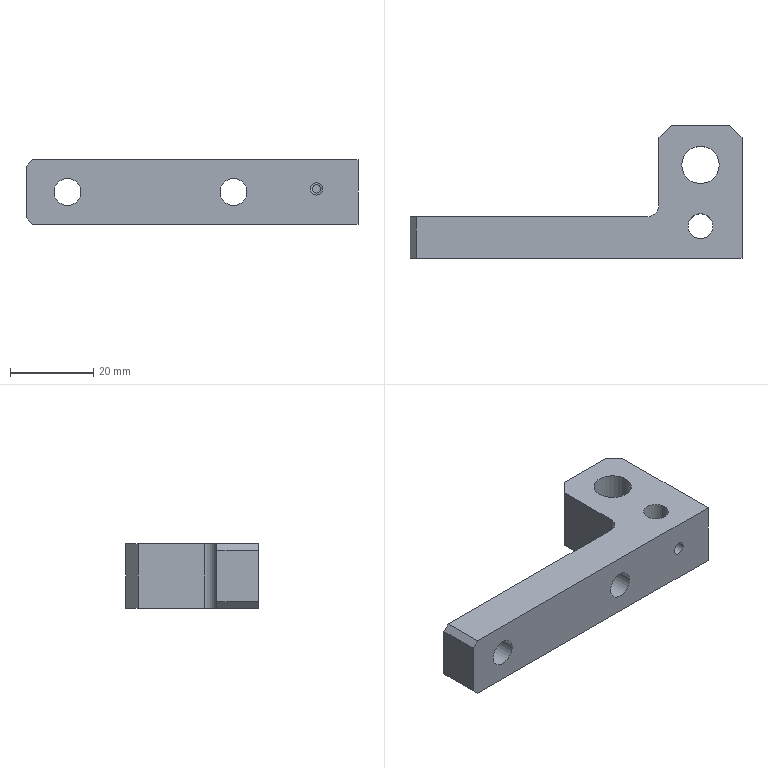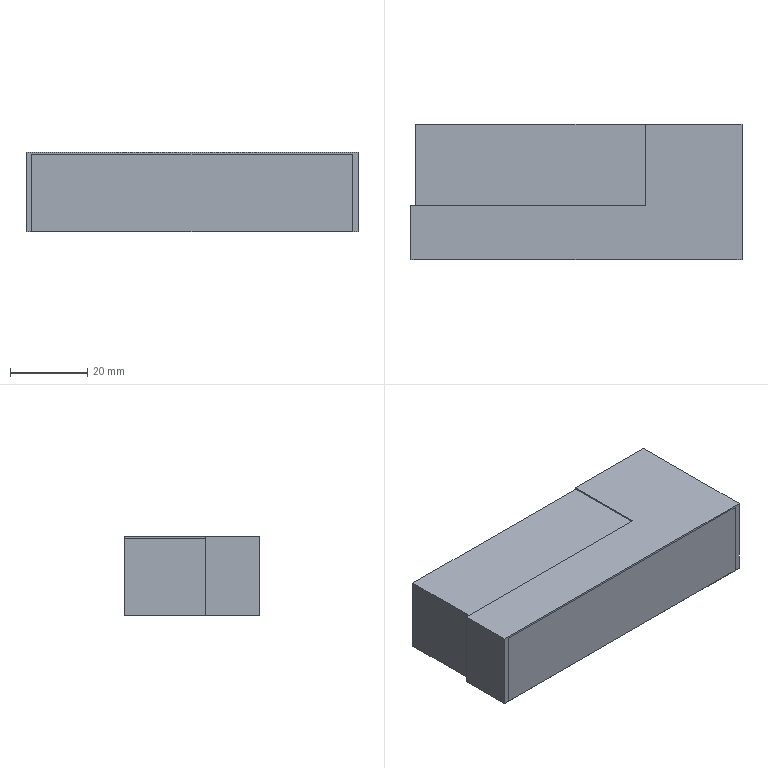CAM job | NX | 3+2 milling, drilling | part box 80 x 32 x 15.5 mm | stock box 86 x 35 x 20.5 mm
Tools:
number,name,description,diameter,corner_radius,flute_length,length,flutes
0,D4-12-D4-50-3T-FINISH,D4-12-D4-50-3T,4.0,0.0,12.0,50.0,3
4,D5-15-D6-50-3T-ROUGH,D5-15-D6-50-3T,5.0,0.0,15.0,16.0,3
6,D6-18-D6-50-3T-FINISH,D6-18-D6-50-3T,6.0,0.0,18.0,50.0,3
1,D10-30-D10-75-3T-ROUGH,D10-30-D10-75-3T-粗,10.0,0.0,30.0,75.0,2
10,D63面刀,D63面刀,63.0,0.0,30.0,30.0,4
2,点孔D10-150-90度,点孔D10-150-90度,10.0,0.0,0.0,150.0,2
0,钻头D2.0-29-55,钻刀D2.0-29-55,2.0,0.0,29.0,55.0,2
0,钻头D3.0-42-71,钻刀D3.0-42-71,3.0,0.0,42.0,71.0,2
7,钻头D5.0-62-92,钻刀D5.0-62-92,5.0,0.0,62.0,92.0,2
15,钻头D6.5-73-105,钻刀D6.5-73-105,6.5,0.0,73.0,105.0,2
8,上排M6-23-D6-63,上排M6-23-D6-63,6.0,0.0,23.0,26.0,2
5,倒角D4-90度,倒角D4-90度,4.0,0.0,5.0,50.0,2
Operations:
program,operation,operation_type,tool,method,geometry_group,spindle_rpm,surface_speed,feed_per_tooth,feed_cut,feed_plunge,cut_length_mm,path_length_mm,cut_time_min,machine_time_min
A1,低壁铣光面,VolumeBased25DMillingOperation,D63面刀,METHOD,WORKPIECE_54,1600.0,316.0,0.0781,500.0,100.0,153.5,187.5,0.307,0.3104
A1,动态粗,CavityMilling,D10-30-D10-75-3T-ROUGH,METHOD,WORKPIECE_54,3500.0,109.0,0.2143,1500.0,100.0,5601.171,5673.171,3.615,3.622
A1,DRILLING,Operation,点孔D10-150-90度,METHOD,WORKPIECE_54,1300.0,40.0,0.0308,80.0,0.0,12.0,82.052,0.15,0.157
A1,DRILLING_1,Operation,钻头D5.0-62-92,METHOD,WORKPIECE_54,1300.0,20.0,0.0231,60.0,0.0,42.0,142.052,0.7,0.71
A1,DRILLING_2,Operation,上排M6-23-D6-63,METHOD,WORKPIECE_54,300.0,5.0,0.0017,1.0,0.0,8.0,56.0,8.0,8.005
A1,PLANAR_MILL_4_COPY,PlanarMilling,D5-15-D6-50-3T-ROUGH,METHOD,WORKPIECE_54,3000.0,47.0,0.0444,400.0,100.0,429.335,489.235,1.073,1.079
A1,PLANAR_MILL_4,PlanarMilling,D5-15-D6-50-3T-ROUGH,METHOD,WORKPIECE_54,3000.0,47.0,0.0444,400.0,100.0,417.724,461.624,1.044,1.049
A1,动态粗_COPY,CavityMilling,D6-18-D6-50-3T-FINISH,METHOD,WORKPIECE_54,3500.0,65.0,0.0762,800.0,100.0,98.613,170.613,0.1233,0.1305,regenerated
A1,PLANAR_MILL_1,PlanarMilling,D6-18-D6-50-3T-FINISH,METHOD,WORKPIECE_54,3000.0,56.0,0.0889,800.0,100.0,761.114,978.488,0.9514,0.9731
A1,PLANAR_MILL_5,PlanarMilling,D4-12-D4-50-3T-FINISH,METHOD,WORKPIECE_54,3000.0,37.0,0.0222,200.0,100.0,1266.953,1311.953,6.335,6.339
A1,PLANAR_MILL_5_COPY,PlanarMilling,D6-18-D6-50-3T-FINISH,METHOD,WORKPIECE_54,3000.0,56.0,0.0333,300.0,100.0,27.259,95.259,0.0909,0.0977
A1,PLANAR_MILL_2,PlanarMilling,倒角D4-90度,METHOD,WORKPIECE_54,3000.0,37.0,0.1333,800.0,100.0,239.506,278.506,0.2994,0.3033
A1,PLANAR_MILL_6_COPY_COPY,PlanarMilling,倒角D4-90度,METHOD,WORKPIECE_54,3000.0,37.0,0.1333,800.0,100.0,21.609,72.609,0.027,0.0321
A1,PLANAR_MILL_6_COPY_COPY_1,PlanarMilling,倒角D4-90度,METHOD,WORKPIECE_54,3000.0,37.0,0.1333,800.0,100.0,39.412,77.412,0.0493,0.0531
A1,PLANAR_MILL_6_COPY,PlanarMilling,倒角D4-90度,METHOD,WORKPIECE_54,3000.0,37.0,0.1333,800.0,100.0,23.132,61.132,0.0289,0.0327
B1,ADAPTIVE_MILLING,CavityMilling,D10-30-D10-75-3T-ROUGH,METHOD,WORKPIECE_55,3000.0,94.0,0.25,1500.0,100.0,8661.796,8695.596,3.43,3.433
B1,PLANAR_MILL_3,PlanarMilling,D63面刀,METHOD,WORKPIECE_55,1600.0,251.0,0.0938,600.0,100.0,155.0,189.0,0.2583,0.2617
B1,PLANAR_MILL_6,PlanarMilling,倒角D4-90度,METHOD,WORKPIECE_55,3000.0,37.0,0.1333,800.0,100.0,238.622,275.622,0.2983,0.302
B1,PLANAR_MILL_6_COPY_1,PlanarMilling,倒角D4-90度,METHOD,WORKPIECE_55,3000.0,37.0,0.1333,800.0,100.0,43.786,137.27,0.0547,0.0641
C1,PLANAR_MILL_7,PlanarMilling,D10-30-D10-75-3T-ROUGH,METHOD,C-G56,3000.0,94.0,0.1333,800.0,100.0,40.243,166.056,0.0503,0.0629
C1,PLANAR_MILL_7_COPY,PlanarMilling,D6-18-D6-50-3T-FINISH,METHOD,C-G56,3000.0,56.0,0.0667,600.0,100.0,32.243,157.914,0.0537,0.0663
C1,DRILLING_3,Operation,点孔D10-150-90度,METHOD,C-G56,1600.0,50.0,0.0187,60.0,0.0,4.0,48.0,0.0667,0.0711
C1,DRILLING_3_COPY_2,Operation,点孔D10-150-90度,METHOD,C-G56,1600.0,50.0,0.0187,60.0,0.0,8.0,99.112,0.1333,0.1424
C1,DRILLING_3_COPY,Operation,钻头D3.0-42-71,METHOD,C-G56,1600.0,15.0,0.0187,60.0,0.0,14.0,68.0,0.2333,0.2387
C1,DRILLING_3_COPY_COPY,Operation,钻头D2.0-29-55,METHOD,C-G56,1600.0,10.0,0.0094,30.0,0.0,23.0,86.0,0.7667,0.773
C1,DRILLING_3_COPY_1,Operation,钻头D6.5-73-105,METHOD,C-G56,1200.0,24.0,0.025,60.0,0.0,32.0,147.112,0.5333,0.5448
C1,DRILLING_3_COPY_3,Operation,点孔D10-150-90度,METHOD,C-G56,1600.0,50.0,0.0187,60.0,0.0,4.5,49.0,0.075,0.0794
C1,DRILLING_3_COPY_2_COPY,Operation,点孔D10-150-90度,METHOD,C-G56,1600.0,50.0,0.0187,60.0,0.0,12.5,108.112,0.2083,0.2179